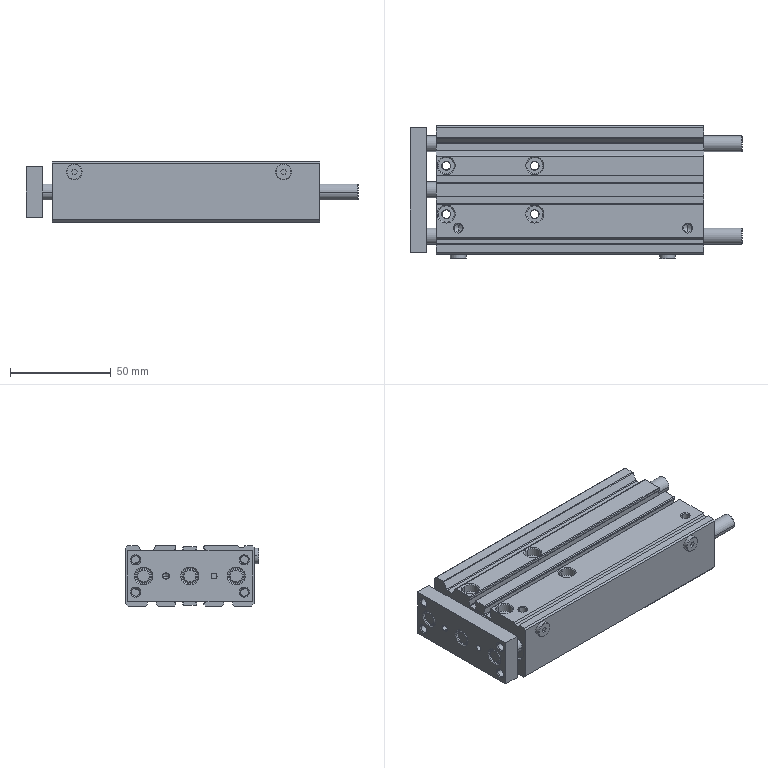Part | STEP file | TCL16x100S_0_ | 2 solids | 413 faces | box 165 x 66.1 x 30 mm | volume 211792 mm3 | cylinder 169 | plane 140 | cone 102 | spline 2 | commonest cylinder face diameters 4.134 x28 8 x26 3 x21 0.8 x20 0.4 x16 4.5 x8